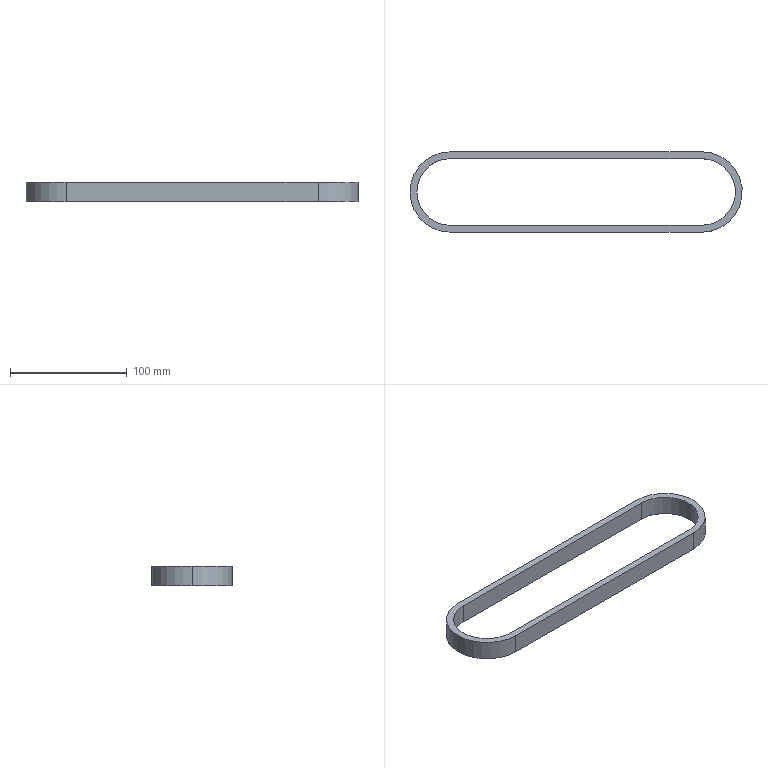Part | SolidWorks | features BaseBody 1 | 1 solid | 12 faces | box 284.87 x 68.87 x 17 mm | volume 63172 mm3 | cylinder 6 | plane 6 | commonest cylinder face diameters 57.07 x3 68.87 x3
STEP:
#1=CARTESIAN_POINT('',(0.,28.535,17.));
#2=VERTEX_POINT('',#1);
#3=CARTESIAN_POINT('',(-28.535,0.,17.));
#4=VERTEX_POINT('',#3);
#5=CARTESIAN_POINT('',(0.,0.,17.));
#6=DIRECTION('',(0.,0.,1.));
#7=DIRECTION('',(1.,0.,0.));
#8=AXIS2_PLACEMENT_3D('',#5,#6,#7);
#9=CIRCLE('',#8,28.535);
#10=EDGE_CURVE('',#2,#4,#9,.T.);
#11=ORIENTED_EDGE('',*,*,#10,.T.);
#12=CARTESIAN_POINT('',(-28.535,0.,0.));
#13=VERTEX_POINT('',#12);
#14=CARTESIAN_POINT('',(-28.535,0.,17.));
#15=DIRECTION('',(0.,0.,-1.));
#16=VECTOR('',#15,1000.);
#17=LINE('',#14,#16);
#18=EDGE_CURVE('',#4,#13,#17,.T.);
#19=ORIENTED_EDGE('',*,*,#18,.T.);
#20=CARTESIAN_POINT('',(0.,28.535,0.));
#21=VERTEX_POINT('',#20);
#22=CARTESIAN_POINT('',(0.,0.,0.));
#23=DIRECTION('',(0.,0.,1.));
#24=DIRECTION('',(1.,0.,0.));
#25=AXIS2_PLACEMENT_3D('',#22,#23,#24);
#26=CIRCLE('',#25,28.535);
#27=EDGE_CURVE('',#21,#13,#26,.T.);
#28=ORIENTED_EDGE('',*,*,#27,.F.);
#29=CARTESIAN_POINT('',(0.,28.535,17.));
#30=DIRECTION('',(0.,0.,-1.));
#31=VECTOR('',#30,1000.);
#32=LINE('',#29,#31);
#33=EDGE_CURVE('',#2,#21,#32,.T.);
#34=ORIENTED_EDGE('',*,*,#33,.F.);
#35=EDGE_LOOP('',(#11,#19,#28,#34));
#36=FACE_OUTER_BOUND('',#35,.T.);
#37=CARTESIAN_POINT('',(0.,0.,17.));
#38=DIRECTION('',(0.,0.,-1.));
#39=DIRECTION('',(-1.,0.,0.));
#40=AXIS2_PLACEMENT_3D('',#37,#38,#39);
#41=CYLINDRICAL_SURFACE('',#40,28.535);
#42=ADVANCED_FACE('',(#36),#41,.F.);
#43=CARTESIAN_POINT('',(-34.435,0.,17.));
#44=VERTEX_POINT('',#43);
#45=CARTESIAN_POINT('',(0.,-34.435,17.));
#46=VERTEX_POINT('',#45);
#47=CARTESIAN_POINT('',(0.,0.,17.));
#48=DIRECTION('',(0.,0.,1.));
#49=DIRECTION('',(1.,0.,0.));
#50=AXIS2_PLACEMENT_3D('',#47,#48,#49);
#51=CIRCLE('',#50,34.435);
#52=EDGE_CURVE('',#44,#46,#51,.T.);
#53=ORIENTED_EDGE('',*,*,#52,.F.);
#54=CARTESIAN_POINT('',(-34.435,0.,0.));
#55=VERTEX_POINT('',#54);
#56=CARTESIAN_POINT('',(-34.435,0.,17.));
#57=DIRECTION('',(0.,0.,-1.));
#58=VECTOR('',#57,1000.);
#59=LINE('',#56,#58);
#60=EDGE_CURVE('',#44,#55,#59,.T.);
#61=ORIENTED_EDGE('',*,*,#60,.T.);
#62=CARTESIAN_POINT('',(0.,-34.435,0.));
#63=VERTEX_POINT('',#62);
#64=CARTESIAN_POINT('',(0.,0.,0.));
#65=DIRECTION('',(0.,0.,1.));
#66=DIRECTION('',(1.,0.,0.));
#67=AXIS2_PLACEMENT_3D('',#64,#65,#66);
#68=CIRCLE('',#67,34.435);
#69=EDGE_CURVE('',#55,#63,#68,.T.);
#70=ORIENTED_EDGE('',*,*,#69,.T.);
#71=CARTESIAN_POINT('',(0.,-34.435,17.));
#72=DIRECTION('',(0.,0.,-1.));
#73=VECTOR('',#72,1000.);
#74=LINE('',#71,#73);
#75=EDGE_CURVE('',#46,#63,#74,.T.);
#76=ORIENTED_EDGE('',*,*,#75,.F.);
#77=EDGE_LOOP('',(#53,#61,#70,#76));
#78=FACE_OUTER_BOUND('',#77,.T.);
#79=CARTESIAN_POINT('',(0.,0.,17.));
#80=DIRECTION('',(0.,0.,-1.));
#81=DIRECTION('',(-1.,0.,0.));
#82=AXIS2_PLACEMENT_3D('',#79,#80,#81);
#83=CYLINDRICAL_SURFACE('',#82,34.435);
#84=ADVANCED_FACE('',(#78),#83,.T.);
#85=CARTESIAN_POINT('',(0.,34.435,17.));
#86=VERTEX_POINT('',#85);
#87=CARTESIAN_POINT('',(0.,0.,17.));
#88=DIRECTION('',(0.,0.,1.));
#89=DIRECTION('',(1.,0.,0.));
#90=AXIS2_PLACEMENT_3D('',#87,#88,#89);
#91=CIRCLE('',#90,34.435);
#92=EDGE_CURVE('',#86,#44,#91,.T.);
#93=ORIENTED_EDGE('',*,*,#92,.T.);
#94=ORIENTED_EDGE('',*,*,#52,.T.);
#95=CARTESIAN_POINT('',(216.,-34.435,17.));
#96=VERTEX_POINT('',#95);
#97=CARTESIAN_POINT('',(0.,-34.435,17.));
#98=DIRECTION('',(1.,0.,0.));
#99=VECTOR('',#98,1000.);
#100=LINE('',#97,#99);
#101=EDGE_CURVE('',#46,#96,#100,.T.);
#102=ORIENTED_EDGE('',*,*,#101,.T.);
#103=CARTESIAN_POINT('',(216.,34.435,17.));
#104=VERTEX_POINT('',#103);
#105=CARTESIAN_POINT('',(216.,0.,17.));
#106=DIRECTION('',(0.,0.,1.));
#107=DIRECTION('',(1.,0.,0.));
#108=AXIS2_PLACEMENT_3D('',#105,#106,#107);
#109=CIRCLE('',#108,34.435);
#110=EDGE_CURVE('',#96,#104,#109,.T.);
#111=ORIENTED_EDGE('',*,*,#110,.T.);
#112=CARTESIAN_POINT('',(0.,34.435,17.));
#113=DIRECTION('',(-1.,0.,0.));
#114=VECTOR('',#113,1000.);
#115=LINE('',#112,#114);
#116=EDGE_CURVE('',#104,#86,#115,.T.);
#117=ORIENTED_EDGE('',*,*,#116,.T.);
#118=EDGE_LOOP('',(#93,#94,#102,#111,#117));
#119=FACE_OUTER_BOUND('',#118,.T.);
#120=CARTESIAN_POINT('',(0.,-28.535,17.));
#121=VERTEX_POINT('',#120);
#122=CARTESIAN_POINT('',(216.,-28.535,17.));
#123=VERTEX_POINT('',#122);
#124=CARTESIAN_POINT('',(0.,-28.535,17.));
#125=DIRECTION('',(1.,0.,0.));
#126=VECTOR('',#125,1000.);
#127=LINE('',#124,#126);
#128=EDGE_CURVE('',#121,#123,#127,.T.);
#129=ORIENTED_EDGE('',*,*,#128,.F.);
#130=CARTESIAN_POINT('',(0.,0.,17.));
#131=DIRECTION('',(0.,0.,1.));
#132=DIRECTION('',(1.,0.,0.));
#133=AXIS2_PLACEMENT_3D('',#130,#131,#132);
#134=CIRCLE('',#133,28.535);
#135=EDGE_CURVE('',#4,#121,#134,.T.);
#136=ORIENTED_EDGE('',*,*,#135,.F.);
#137=ORIENTED_EDGE('',*,*,#10,.F.);
#138=CARTESIAN_POINT('',(216.,28.535,17.));
#139=VERTEX_POINT('',#138);
#140=CARTESIAN_POINT('',(0.,28.535,17.));
#141=DIRECTION('',(-1.,0.,0.));
#142=VECTOR('',#141,1000.);
#143=LINE('',#140,#142);
#144=EDGE_CURVE('',#139,#2,#143,.T.);
#145=ORIENTED_EDGE('',*,*,#144,.F.);
#146=CARTESIAN_POINT('',(216.,0.,17.));
#147=DIRECTION('',(0.,0.,1.));
#148=DIRECTION('',(1.,0.,0.));
#149=AXIS2_PLACEMENT_3D('',#146,#147,#148);
#150=CIRCLE('',#149,28.535);
#151=EDGE_CURVE('',#123,#139,#150,.T.);
#152=ORIENTED_EDGE('',*,*,#151,.F.);
#153=EDGE_LOOP('',(#129,#136,#137,#145,#152));
#154=FACE_BOUND('',#153,.T.);
#155=CARTESIAN_POINT('',(0.,0.,17.));
#156=DIRECTION('',(0.,0.,1.));
#157=DIRECTION('',(1.,0.,0.));
#158=AXIS2_PLACEMENT_3D('',#155,#156,#157);
#159=PLANE('',#158);
#160=ADVANCED_FACE('',(#119,#154),#159,.T.);
#161=CARTESIAN_POINT('',(0.,34.435,0.));
#162=VERTEX_POINT('',#161);
#163=CARTESIAN_POINT('',(0.,0.,0.));
#164=DIRECTION('',(0.,0.,1.));
#165=DIRECTION('',(1.,0.,0.));
#166=AXIS2_PLACEMENT_3D('',#163,#164,#165);
#167=CIRCLE('',#166,34.435);
#168=EDGE_CURVE('',#162,#55,#167,.T.);
#169=ORIENTED_EDGE('',*,*,#168,.F.);
#170=CARTESIAN_POINT('',(216.,34.435,0.));
#171=VERTEX_POINT('',#170);
#172=CARTESIAN_POINT('',(0.,34.435,0.));
#173=DIRECTION('',(-1.,0.,0.));
#174=VECTOR('',#173,1000.);
#175=LINE('',#172,#174);
#176=EDGE_CURVE('',#171,#162,#175,.T.);
#177=ORIENTED_EDGE('',*,*,#176,.F.);
#178=CARTESIAN_POINT('',(216.,-34.435,0.));
#179=VERTEX_POINT('',#178);
#180=CARTESIAN_POINT('',(216.,0.,0.));
#181=DIRECTION('',(0.,0.,1.));
#182=DIRECTION('',(1.,0.,0.));
#183=AXIS2_PLACEMENT_3D('',#180,#181,#182);
#184=CIRCLE('',#183,34.435);
#185=EDGE_CURVE('',#179,#171,#184,.T.);
#186=ORIENTED_EDGE('',*,*,#185,.F.);
#187=CARTESIAN_POINT('',(0.,-34.435,0.));
#188=DIRECTION('',(1.,0.,0.));
#189=VECTOR('',#188,1000.);
#190=LINE('',#187,#189);
#191=EDGE_CURVE('',#63,#179,#190,.T.);
#192=ORIENTED_EDGE('',*,*,#191,.F.);
#193=ORIENTED_EDGE('',*,*,#69,.F.);
#194=EDGE_LOOP('',(#169,#177,#186,#192,#193));
#195=FACE_OUTER_BOUND('',#194,.T.);
#196=ORIENTED_EDGE('',*,*,#27,.T.);
#197=CARTESIAN_POINT('',(0.,-28.535,0.));
#198=VERTEX_POINT('',#197);
#199=CARTESIAN_POINT('',(0.,0.,0.));
#200=DIRECTION('',(0.,0.,1.));
#201=DIRECTION('',(1.,0.,0.));
#202=AXIS2_PLACEMENT_3D('',#199,#200,#201);
#203=CIRCLE('',#202,28.535);
#204=EDGE_CURVE('',#13,#198,#203,.T.);
#205=ORIENTED_EDGE('',*,*,#204,.T.);
#206=CARTESIAN_POINT('',(216.,-28.535,0.));
#207=VERTEX_POINT('',#206);
#208=CARTESIAN_POINT('',(0.,-28.535,0.));
#209=DIRECTION('',(1.,0.,0.));
#210=VECTOR('',#209,1000.);
#211=LINE('',#208,#210);
#212=EDGE_CURVE('',#198,#207,#211,.T.);
#213=ORIENTED_EDGE('',*,*,#212,.T.);
#214=CARTESIAN_POINT('',(216.,28.535,0.));
#215=VERTEX_POINT('',#214);
#216=CARTESIAN_POINT('',(216.,0.,0.));
#217=DIRECTION('',(0.,0.,1.));
#218=DIRECTION('',(1.,0.,0.));
#219=AXIS2_PLACEMENT_3D('',#216,#217,#218);
#220=CIRCLE('',#219,28.535);
#221=EDGE_CURVE('',#207,#215,#220,.T.);
#222=ORIENTED_EDGE('',*,*,#221,.T.);
#223=CARTESIAN_POINT('',(0.,28.535,0.));
#224=DIRECTION('',(-1.,0.,0.));
#225=VECTOR('',#224,1000.);
#226=LINE('',#223,#225);
#227=EDGE_CURVE('',#215,#21,#226,.T.);
#228=ORIENTED_EDGE('',*,*,#227,.T.);
#229=EDGE_LOOP('',(#196,#205,#213,#222,#228));
#230=FACE_BOUND('',#229,.T.);
#231=CARTESIAN_POINT('',(0.,0.,0.));
#232=DIRECTION('',(0.,0.,1.));
#233=DIRECTION('',(1.,0.,0.));
#234=AXIS2_PLACEMENT_3D('',#231,#232,#233);
#235=PLANE('',#234);
#236=ADVANCED_FACE('',(#195,#230),#235,.F.);
#237=ORIENTED_EDGE('',*,*,#60,.F.);
#238=ORIENTED_EDGE('',*,*,#92,.F.);
#239=CARTESIAN_POINT('',(0.,34.435,17.));
#240=DIRECTION('',(0.,0.,-1.));
#241=VECTOR('',#240,1000.);
#242=LINE('',#239,#241);
#243=EDGE_CURVE('',#86,#162,#242,.T.);
#244=ORIENTED_EDGE('',*,*,#243,.T.);
#245=ORIENTED_EDGE('',*,*,#168,.T.);
#246=EDGE_LOOP('',(#237,#238,#244,#245));
#247=FACE_OUTER_BOUND('',#246,.T.);
#248=CARTESIAN_POINT('',(0.,0.,17.));
#249=DIRECTION('',(0.,0.,-1.));
#250=DIRECTION('',(-1.,0.,0.));
#251=AXIS2_PLACEMENT_3D('',#248,#249,#250);
#252=CYLINDRICAL_SURFACE('',#251,34.435);
#253=ADVANCED_FACE('',(#247),#252,.T.);
#254=ORIENTED_EDGE('',*,*,#191,.T.);
#255=CARTESIAN_POINT('',(216.,-34.435,17.));
#256=DIRECTION('',(0.,0.,-1.));
#257=VECTOR('',#256,1000.);
#258=LINE('',#255,#257);
#259=EDGE_CURVE('',#96,#179,#258,.T.);
#260=ORIENTED_EDGE('',*,*,#259,.F.);
#261=ORIENTED_EDGE('',*,*,#101,.F.);
#262=ORIENTED_EDGE('',*,*,#75,.T.);
#263=EDGE_LOOP('',(#254,#260,#261,#262));
#264=FACE_OUTER_BOUND('',#263,.T.);
#265=CARTESIAN_POINT('',(0.,-34.435,17.));
#266=DIRECTION('',(0.,1.,0.));
#267=DIRECTION('',(0.,0.,1.));
#268=AXIS2_PLACEMENT_3D('',#265,#266,#267);
#269=PLANE('',#268);
#270=ADVANCED_FACE('',(#264),#269,.F.);
#271=ORIENTED_EDGE('',*,*,#185,.T.);
#272=CARTESIAN_POINT('',(216.,34.435,17.));
#273=DIRECTION('',(0.,0.,-1.));
#274=VECTOR('',#273,1000.);
#275=LINE('',#272,#274);
#276=EDGE_CURVE('',#104,#171,#275,.T.);
#277=ORIENTED_EDGE('',*,*,#276,.F.);
#278=ORIENTED_EDGE('',*,*,#110,.F.);
#279=ORIENTED_EDGE('',*,*,#259,.T.);
#280=EDGE_LOOP('',(#271,#277,#278,#279));
#281=FACE_OUTER_BOUND('',#280,.T.);
#282=CARTESIAN_POINT('',(216.,0.,17.));
#283=DIRECTION('',(0.,0.,-1.));
#284=DIRECTION('',(-1.,0.,0.));
#285=AXIS2_PLACEMENT_3D('',#282,#283,#284);
#286=CYLINDRICAL_SURFACE('',#285,34.435);
#287=ADVANCED_FACE('',(#281),#286,.T.);
#288=ORIENTED_EDGE('',*,*,#176,.T.);
#289=ORIENTED_EDGE('',*,*,#243,.F.);
#290=ORIENTED_EDGE('',*,*,#116,.F.);
#291=ORIENTED_EDGE('',*,*,#276,.T.);
#292=EDGE_LOOP('',(#288,#289,#290,#291));
#293=FACE_OUTER_BOUND('',#292,.T.);
#294=CARTESIAN_POINT('',(0.,34.435,17.));
#295=DIRECTION('',(0.,-1.,0.));
#296=DIRECTION('',(0.,0.,-1.));
#297=AXIS2_PLACEMENT_3D('',#294,#295,#296);
#298=PLANE('',#297);
#299=ADVANCED_FACE('',(#293),#298,.F.);
#300=ORIENTED_EDGE('',*,*,#18,.F.);
#301=ORIENTED_EDGE('',*,*,#135,.T.);
#302=CARTESIAN_POINT('',(0.,-28.535,17.));
#303=DIRECTION('',(0.,0.,-1.));
#304=VECTOR('',#303,1000.);
#305=LINE('',#302,#304);
#306=EDGE_CURVE('',#121,#198,#305,.T.);
#307=ORIENTED_EDGE('',*,*,#306,.T.);
#308=ORIENTED_EDGE('',*,*,#204,.F.);
#309=EDGE_LOOP('',(#300,#301,#307,#308));
#310=FACE_OUTER_BOUND('',#309,.T.);
#311=CARTESIAN_POINT('',(0.,0.,17.));
#312=DIRECTION('',(0.,0.,-1.));
#313=DIRECTION('',(-1.,0.,0.));
#314=AXIS2_PLACEMENT_3D('',#311,#312,#313);
#315=CYLINDRICAL_SURFACE('',#314,28.535);
#316=ADVANCED_FACE('',(#310),#315,.F.);
#317=ORIENTED_EDGE('',*,*,#212,.F.);
#318=ORIENTED_EDGE('',*,*,#306,.F.);
#319=ORIENTED_EDGE('',*,*,#128,.T.);
#320=CARTESIAN_POINT('',(216.,-28.535,17.));
#321=DIRECTION('',(0.,0.,-1.));
#322=VECTOR('',#321,1000.);
#323=LINE('',#320,#322);
#324=EDGE_CURVE('',#123,#207,#323,.T.);
#325=ORIENTED_EDGE('',*,*,#324,.T.);
#326=EDGE_LOOP('',(#317,#318,#319,#325));
#327=FACE_OUTER_BOUND('',#326,.T.);
#328=CARTESIAN_POINT('',(0.,-28.535,17.));
#329=DIRECTION('',(0.,1.,0.));
#330=DIRECTION('',(-1.,0.,0.));
#331=AXIS2_PLACEMENT_3D('',#328,#329,#330);
#332=PLANE('',#331);
#333=ADVANCED_FACE('',(#327),#332,.T.);
#334=ORIENTED_EDGE('',*,*,#221,.F.);
#335=ORIENTED_EDGE('',*,*,#324,.F.);
#336=ORIENTED_EDGE('',*,*,#151,.T.);
#337=CARTESIAN_POINT('',(216.,28.535,17.));
#338=DIRECTION('',(0.,0.,-1.));
#339=VECTOR('',#338,1000.);
#340=LINE('',#337,#339);
#341=EDGE_CURVE('',#139,#215,#340,.T.);
#342=ORIENTED_EDGE('',*,*,#341,.T.);
#343=EDGE_LOOP('',(#334,#335,#336,#342));
#344=FACE_OUTER_BOUND('',#343,.T.);
#345=CARTESIAN_POINT('',(216.,0.,17.));
#346=DIRECTION('',(0.,0.,-1.));
#347=DIRECTION('',(-1.,0.,0.));
#348=AXIS2_PLACEMENT_3D('',#345,#346,#347);
#349=CYLINDRICAL_SURFACE('',#348,28.535);
#350=ADVANCED_FACE('',(#344),#349,.F.);
#351=ORIENTED_EDGE('',*,*,#227,.F.);
#352=ORIENTED_EDGE('',*,*,#341,.F.);
#353=ORIENTED_EDGE('',*,*,#144,.T.);
#354=ORIENTED_EDGE('',*,*,#33,.T.);
#355=EDGE_LOOP('',(#351,#352,#353,#354));
#356=FACE_OUTER_BOUND('',#355,.T.);
#357=CARTESIAN_POINT('',(0.,28.535,17.));
#358=DIRECTION('',(0.,-1.,0.));
#359=DIRECTION('',(1.,0.,0.));
#360=AXIS2_PLACEMENT_3D('',#357,#358,#359);
#361=PLANE('',#360);
#362=ADVANCED_FACE('',(#356),#361,.T.);
#363=CLOSED_SHELL('',(#42,#84,#160,#236,#253,#270,#287,#299,#316,#333,#350,#362));
#364=MANIFOLD_SOLID_BREP('',#363);
#365=CARTESIAN_POINT('',(0.,0.,0.));
#366=DIRECTION('',(0.,0.,1.));
#367=DIRECTION('',(1.,0.,0.));
#368=AXIS2_PLACEMENT_3D('',#365,#366,#367);
#369=(LENGTH_UNIT()NAMED_UNIT(*)SI_UNIT(.MILLI.,.METRE.));
#370=UNCERTAINTY_MEASURE_WITH_UNIT(LENGTH_MEASURE(0.00001),#369,'','');
#371=(NAMED_UNIT(*)PLANE_ANGLE_UNIT()SI_UNIT($,.RADIAN.));
#372=(NAMED_UNIT(*)SI_UNIT($,.STERADIAN.)SOLID_ANGLE_UNIT());
#373=(GEOMETRIC_REPRESENTATION_CONTEXT(3)GLOBAL_UNCERTAINTY_ASSIGNED_CONTEXT((#370))GLOBAL_UNIT_ASSIGNED_CONTEXT((#369,#371,#372))REPRESENTATION_CONTEXT('',''));
#374=ADVANCED_BREP_SHAPE_REPRESENTATION('',(#364,#368),#373);